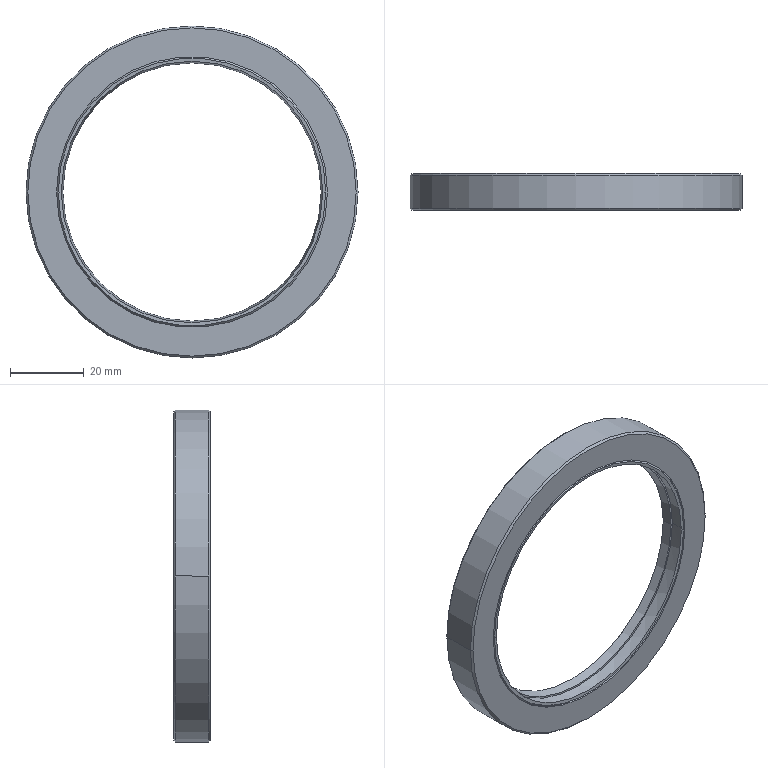Part | SolidWorks | features BaseBody 1 | 1 solid | 37 faces | box 90 x 10 x 90 mm | volume 7063 mm3 | cone 20 | cylinder 8 | plane 5 | spline 4 | commonest cylinder face diameters 73.436 x4 88 x2 90 x2
STEP:
#1=CARTESIAN_POINT('',(36.965,3.733,0.));
#2=VERTEX_POINT('',#1);
#3=CARTESIAN_POINT('',(-36.965,3.733,0.));
#4=VERTEX_POINT('',#3);
#5=CARTESIAN_POINT('',(0.,3.733,0.));
#6=DIRECTION('',(0.,1.,0.));
#7=DIRECTION('',(-1.,0.,0.));
#8=AXIS2_PLACEMENT_3D('',#5,#6,#7);
#9=CIRCLE('',#8,36.965);
#10=EDGE_CURVE('',#2,#4,#9,.T.);
#11=ORIENTED_EDGE('',*,*,#10,.F.);
#12=CARTESIAN_POINT('',(36.518,3.286,0.));
#13=VERTEX_POINT('',#12);
#14=CARTESIAN_POINT('',(36.518,3.733,0.));
#15=DIRECTION('',(0.,0.,-1.));
#16=DIRECTION('',(1.,0.,0.));
#17=AXIS2_PLACEMENT_3D('',#14,#15,#16);
#18=CIRCLE('',#17,0.4472);
#19=EDGE_CURVE('',#2,#13,#18,.T.);
#20=ORIENTED_EDGE('',*,*,#19,.T.);
#21=CARTESIAN_POINT('',(-36.518,3.286,0.));
#22=VERTEX_POINT('',#21);
#23=CARTESIAN_POINT('',(0.,3.286,0.));
#24=DIRECTION('',(0.,-1.,0.));
#25=DIRECTION('',(1.,0.,0.));
#26=AXIS2_PLACEMENT_3D('',#23,#24,#25);
#27=CIRCLE('',#26,36.518);
#28=EDGE_CURVE('',#22,#13,#27,.T.);
#29=ORIENTED_EDGE('',*,*,#28,.F.);
#30=CARTESIAN_POINT('',(-36.518,3.733,0.));
#31=DIRECTION('',(0.,0.,1.));
#32=DIRECTION('',(-1.,0.,0.));
#33=AXIS2_PLACEMENT_3D('',#30,#31,#32);
#34=CIRCLE('',#33,0.4472);
#35=EDGE_CURVE('',#4,#22,#34,.T.);
#36=ORIENTED_EDGE('',*,*,#35,.F.);
#37=EDGE_LOOP('',(#11,#20,#29,#36));
#38=FACE_OUTER_BOUND('',#37,.T.);
#39=CARTESIAN_POINT('',(36.965,3.733,0.));
#40=CARTESIAN_POINT('',(36.965,3.733,-73.93));
#41=CARTESIAN_POINT('',(-36.965,3.733,-73.93));
#42=CARTESIAN_POINT('',(-36.965,3.733,0.));
#43=CARTESIAN_POINT('',(36.965,3.471,0.));
#44=CARTESIAN_POINT('',(36.965,3.471,-73.93));
#45=CARTESIAN_POINT('',(-36.965,3.471,-73.93));
#46=CARTESIAN_POINT('',(-36.965,3.471,0.));
#47=CARTESIAN_POINT('',(36.78,3.286,0.));
#48=CARTESIAN_POINT('',(36.78,3.286,-73.56));
#49=CARTESIAN_POINT('',(-36.78,3.286,-73.56));
#50=CARTESIAN_POINT('',(-36.78,3.286,0.));
#51=CARTESIAN_POINT('',(36.518,3.286,0.));
#52=CARTESIAN_POINT('',(36.518,3.286,-73.036));
#53=CARTESIAN_POINT('',(-36.518,3.286,-73.036));
#54=CARTESIAN_POINT('',(-36.518,3.286,0.));
#55=(BOUNDED_SURFACE()B_SPLINE_SURFACE(3,3,((#39,#40,#41,#42),(#43,#44,#45,#46),(#47,#48,#49,#50),(#51,#52,#53,#54)),.UNSPECIFIED.,.F.,.F.,.F.)B_SPLINE_SURFACE_WITH_KNOTS((4,4),(4,4),(0.,1.),(0.,1.),.UNSPECIFIED.)GEOMETRIC_REPRESENTATION_ITEM()RATIONAL_B_SPLINE_SURFACE(((1.,0.3333,0.3333,1.),(0.8047,0.2682,0.2682,0.8047),(0.8047,0.2682,0.2682,0.8047),(1.,0.3333,0.3333,1.)))REPRESENTATION_ITEM('')SURFACE());
#56=ADVANCED_FACE('',(#38),#55,.T.);
#57=CARTESIAN_POINT('',(-36.718,4.133,0.));
#58=VERTEX_POINT('',#57);
#59=CARTESIAN_POINT('',(36.718,4.133,0.));
#60=VERTEX_POINT('',#59);
#61=CARTESIAN_POINT('',(0.,4.133,0.));
#62=DIRECTION('',(0.,-1.,0.));
#63=DIRECTION('',(-1.,0.,0.));
#64=AXIS2_PLACEMENT_3D('',#61,#62,#63);
#65=CIRCLE('',#64,36.718);
#66=EDGE_CURVE('',#58,#60,#65,.T.);
#67=ORIENTED_EDGE('',*,*,#66,.T.);
#68=CARTESIAN_POINT('',(36.518,3.733,0.));
#69=DIRECTION('',(0.,0.,-1.));
#70=DIRECTION('',(1.,0.,0.));
#71=AXIS2_PLACEMENT_3D('',#68,#69,#70);
#72=CIRCLE('',#71,0.4472);
#73=EDGE_CURVE('',#60,#2,#72,.T.);
#74=ORIENTED_EDGE('',*,*,#73,.T.);
#75=ORIENTED_EDGE('',*,*,#10,.T.);
#76=CARTESIAN_POINT('',(-36.518,3.733,0.));
#77=DIRECTION('',(0.,0.,1.));
#78=DIRECTION('',(-1.,0.,0.));
#79=AXIS2_PLACEMENT_3D('',#76,#77,#78);
#80=CIRCLE('',#79,0.4472);
#81=EDGE_CURVE('',#58,#4,#80,.T.);
#82=ORIENTED_EDGE('',*,*,#81,.F.);
#83=EDGE_LOOP('',(#67,#74,#75,#82));
#84=FACE_OUTER_BOUND('',#83,.T.);
#85=CARTESIAN_POINT('',(36.718,4.133,0.));
#86=CARTESIAN_POINT('',(36.718,4.133,-73.436));
#87=CARTESIAN_POINT('',(-36.718,4.133,-73.436));
#88=CARTESIAN_POINT('',(-36.718,4.133,0.));
#89=CARTESIAN_POINT('',(36.873,4.055,0.));
#90=CARTESIAN_POINT('',(36.873,4.055,-73.747));
#91=CARTESIAN_POINT('',(-36.873,4.055,-73.747));
#92=CARTESIAN_POINT('',(-36.873,4.055,0.));
#93=CARTESIAN_POINT('',(36.965,3.907,0.));
#94=CARTESIAN_POINT('',(36.965,3.907,-73.93));
#95=CARTESIAN_POINT('',(-36.965,3.907,-73.93));
#96=CARTESIAN_POINT('',(-36.965,3.907,0.));
#97=CARTESIAN_POINT('',(36.965,3.733,0.));
#98=CARTESIAN_POINT('',(36.965,3.733,-73.93));
#99=CARTESIAN_POINT('',(-36.965,3.733,-73.93));
#100=CARTESIAN_POINT('',(-36.965,3.733,0.));
#101=(BOUNDED_SURFACE()B_SPLINE_SURFACE(3,3,((#85,#86,#87,#88),(#89,#90,#91,#92),(#93,#94,#95,#96),(#97,#98,#99,#100)),.UNSPECIFIED.,.F.,.F.,.T.)B_SPLINE_SURFACE_WITH_KNOTS((4,4),(4,4),(0.,1.),(0.,1.),.UNSPECIFIED.)GEOMETRIC_REPRESENTATION_ITEM()RATIONAL_B_SPLINE_SURFACE(((1.,0.3333,0.3333,1.),(0.9004,0.3001,0.3001,0.9004),(0.9004,0.3001,0.3001,0.9004),(1.,0.3333,0.3333,1.)))REPRESENTATION_ITEM('')SURFACE());
#102=ADVANCED_FACE('',(#84),#101,.T.);
#103=CARTESIAN_POINT('',(44.5,0.,0.));
#104=VERTEX_POINT('',#103);
#105=CARTESIAN_POINT('',(-44.5,0.,0.));
#106=VERTEX_POINT('',#105);
#107=CARTESIAN_POINT('',(0.,0.,0.));
#108=DIRECTION('',(0.,-1.,0.));
#109=DIRECTION('',(-1.,0.,0.));
#110=AXIS2_PLACEMENT_3D('',#107,#108,#109);
#111=CIRCLE('',#110,44.5);
#112=EDGE_CURVE('',#104,#106,#111,.T.);
#113=ORIENTED_EDGE('',*,*,#112,.F.);
#114=CARTESIAN_POINT('',(45.,0.5,0.));
#115=VERTEX_POINT('',#114);
#116=CARTESIAN_POINT('',(45.,0.5,0.));
#117=DIRECTION('',(0.7071,0.7071,0.));
#118=VECTOR('',#117,1000.);
#119=LINE('',#116,#118);
#120=EDGE_CURVE('',#104,#115,#119,.T.);
#121=ORIENTED_EDGE('',*,*,#120,.T.);
#122=CARTESIAN_POINT('',(-45.,0.5,0.));
#123=VERTEX_POINT('',#122);
#124=CARTESIAN_POINT('',(0.,0.5,0.));
#125=DIRECTION('',(0.,-1.,0.));
#126=DIRECTION('',(-1.,0.,0.));
#127=AXIS2_PLACEMENT_3D('',#124,#125,#126);
#128=CIRCLE('',#127,45.);
#129=EDGE_CURVE('',#115,#123,#128,.T.);
#130=ORIENTED_EDGE('',*,*,#129,.T.);
#131=CARTESIAN_POINT('',(-45.,0.5,0.));
#132=DIRECTION('',(-0.7071,0.7071,0.));
#133=VECTOR('',#132,1000.);
#134=LINE('',#131,#133);
#135=EDGE_CURVE('',#106,#123,#134,.T.);
#136=ORIENTED_EDGE('',*,*,#135,.F.);
#137=EDGE_LOOP('',(#113,#121,#130,#136));
#138=FACE_OUTER_BOUND('',#137,.T.);
#139=CARTESIAN_POINT('',(0.,0.5,0.));
#140=DIRECTION('',(0.,1.,0.));
#141=DIRECTION('',(-1.,0.,0.));
#142=AXIS2_PLACEMENT_3D('',#139,#140,#141);
#143=CONICAL_SURFACE('',#142,45.,0.7854);
#144=ADVANCED_FACE('',(#138),#143,.T.);
#145=CARTESIAN_POINT('',(36.718,0.,0.));
#146=VERTEX_POINT('',#145);
#147=CARTESIAN_POINT('',(-36.718,0.,0.));
#148=VERTEX_POINT('',#147);
#149=CARTESIAN_POINT('',(0.,0.,0.));
#150=DIRECTION('',(0.,1.,0.));
#151=DIRECTION('',(-1.,0.,0.));
#152=AXIS2_PLACEMENT_3D('',#149,#150,#151);
#153=CIRCLE('',#152,36.718);
#154=EDGE_CURVE('',#146,#148,#153,.T.);
#155=ORIENTED_EDGE('',*,*,#154,.F.);
#156=CARTESIAN_POINT('',(36.718,0.5,0.));
#157=VERTEX_POINT('',#156);
#158=CARTESIAN_POINT('',(36.718,5.977,0.));
#159=DIRECTION('',(0.,1.,0.));
#160=VECTOR('',#159,1000.);
#161=LINE('',#158,#160);
#162=EDGE_CURVE('',#146,#157,#161,.T.);
#163=ORIENTED_EDGE('',*,*,#162,.T.);
#164=CARTESIAN_POINT('',(-36.718,0.5,0.));
#165=VERTEX_POINT('',#164);
#166=CARTESIAN_POINT('',(0.,0.5,0.));
#167=DIRECTION('',(0.,-1.,0.));
#168=DIRECTION('',(-1.,0.,0.));
#169=AXIS2_PLACEMENT_3D('',#166,#167,#168);
#170=CIRCLE('',#169,36.718);
#171=EDGE_CURVE('',#165,#157,#170,.T.);
#172=ORIENTED_EDGE('',*,*,#171,.F.);
#173=CARTESIAN_POINT('',(-36.718,5.977,0.));
#174=DIRECTION('',(0.,1.,0.));
#175=VECTOR('',#174,1000.);
#176=LINE('',#173,#175);
#177=EDGE_CURVE('',#148,#165,#176,.T.);
#178=ORIENTED_EDGE('',*,*,#177,.F.);
#179=EDGE_LOOP('',(#155,#163,#172,#178));
#180=FACE_OUTER_BOUND('',#179,.T.);
#181=CARTESIAN_POINT('',(0.,5.977,0.));
#182=DIRECTION('',(0.,1.,0.));
#183=DIRECTION('',(-1.,0.,0.));
#184=AXIS2_PLACEMENT_3D('',#181,#182,#183);
#185=CYLINDRICAL_SURFACE('',#184,36.718);
#186=ADVANCED_FACE('',(#180),#185,.F.);
#187=ORIENTED_EDGE('',*,*,#129,.F.);
#188=CARTESIAN_POINT('',(45.,9.5,0.));
#189=VERTEX_POINT('',#188);
#190=CARTESIAN_POINT('',(45.,5.977,0.));
#191=DIRECTION('',(0.,1.,0.));
#192=VECTOR('',#191,1000.);
#193=LINE('',#190,#192);
#194=EDGE_CURVE('',#115,#189,#193,.T.);
#195=ORIENTED_EDGE('',*,*,#194,.T.);
#196=CARTESIAN_POINT('',(-45.,9.5,0.));
#197=VERTEX_POINT('',#196);
#198=CARTESIAN_POINT('',(0.,9.5,0.));
#199=DIRECTION('',(0.,-1.,0.));
#200=DIRECTION('',(-1.,0.,0.));
#201=AXIS2_PLACEMENT_3D('',#198,#199,#200);
#202=CIRCLE('',#201,45.);
#203=EDGE_CURVE('',#189,#197,#202,.T.);
#204=ORIENTED_EDGE('',*,*,#203,.T.);
#205=CARTESIAN_POINT('',(-45.,5.977,0.));
#206=DIRECTION('',(0.,1.,0.));
#207=VECTOR('',#206,1000.);
#208=LINE('',#205,#207);
#209=EDGE_CURVE('',#123,#197,#208,.T.);
#210=ORIENTED_EDGE('',*,*,#209,.F.);
#211=EDGE_LOOP('',(#187,#195,#204,#210));
#212=FACE_OUTER_BOUND('',#211,.T.);
#213=CARTESIAN_POINT('',(0.,5.977,0.));
#214=DIRECTION('',(0.,1.,0.));
#215=DIRECTION('',(-1.,0.,0.));
#216=AXIS2_PLACEMENT_3D('',#213,#214,#215);
#217=CYLINDRICAL_SURFACE('',#216,45.);
#218=ADVANCED_FACE('',(#212),#217,.T.);
#219=CARTESIAN_POINT('',(-36.26,0.,0.));
#220=VERTEX_POINT('',#219);
#221=CARTESIAN_POINT('',(36.26,0.,0.));
#222=VERTEX_POINT('',#221);
#223=CARTESIAN_POINT('',(0.,0.,0.));
#224=DIRECTION('',(0.,1.,0.));
#225=DIRECTION('',(-1.,0.,0.));
#226=AXIS2_PLACEMENT_3D('',#223,#224,#225);
#227=CIRCLE('',#226,36.26);
#228=EDGE_CURVE('',#220,#222,#227,.T.);
#229=ORIENTED_EDGE('',*,*,#228,.T.);
#230=CARTESIAN_POINT('',(36.718,0.5,0.));
#231=DIRECTION('',(0.6756,0.7373,0.));
#232=VECTOR('',#231,1000.);
#233=LINE('',#230,#232);
#234=EDGE_CURVE('',#222,#157,#233,.T.);
#235=ORIENTED_EDGE('',*,*,#234,.T.);
#236=CARTESIAN_POINT('',(0.,0.5,0.));
#237=DIRECTION('',(0.,-1.,0.));
#238=DIRECTION('',(-1.,0.,0.));
#239=AXIS2_PLACEMENT_3D('',#236,#237,#238);
#240=CIRCLE('',#239,36.718);
#241=EDGE_CURVE('',#157,#165,#240,.T.);
#242=ORIENTED_EDGE('',*,*,#241,.T.);
#243=CARTESIAN_POINT('',(-36.718,0.5,0.));
#244=DIRECTION('',(-0.6756,0.7373,0.));
#245=VECTOR('',#244,1000.);
#246=LINE('',#243,#245);
#247=EDGE_CURVE('',#220,#165,#246,.T.);
#248=ORIENTED_EDGE('',*,*,#247,.F.);
#249=EDGE_LOOP('',(#229,#235,#242,#248));
#250=FACE_OUTER_BOUND('',#249,.T.);
#251=CARTESIAN_POINT('',(0.,0.5,0.));
#252=DIRECTION('',(0.,1.,0.));
#253=DIRECTION('',(-1.,0.,0.));
#254=AXIS2_PLACEMENT_3D('',#251,#252,#253);
#255=CONICAL_SURFACE('',#254,36.718,0.7418);
#256=ADVANCED_FACE('',(#250),#255,.T.);
#257=CARTESIAN_POINT('',(44.5,10.,0.));
#258=VERTEX_POINT('',#257);
#259=CARTESIAN_POINT('',(-44.5,10.,0.));
#260=VERTEX_POINT('',#259);
#261=CARTESIAN_POINT('',(0.,10.,0.));
#262=DIRECTION('',(0.,-1.,0.));
#263=DIRECTION('',(1.,0.,0.));
#264=AXIS2_PLACEMENT_3D('',#261,#262,#263);
#265=CIRCLE('',#264,44.5);
#266=EDGE_CURVE('',#258,#260,#265,.T.);
#267=ORIENTED_EDGE('',*,*,#266,.T.);
#268=CARTESIAN_POINT('',(-45.,9.5,0.));
#269=DIRECTION('',(-0.7071,-0.7071,0.));
#270=VECTOR('',#269,1000.);
#271=LINE('',#268,#270);
#272=EDGE_CURVE('',#260,#197,#271,.T.);
#273=ORIENTED_EDGE('',*,*,#272,.T.);
#274=ORIENTED_EDGE('',*,*,#203,.F.);
#275=CARTESIAN_POINT('',(45.,9.5,0.));
#276=DIRECTION('',(0.7071,-0.7071,0.));
#277=VECTOR('',#276,1000.);
#278=LINE('',#275,#277);
#279=EDGE_CURVE('',#258,#189,#278,.T.);
#280=ORIENTED_EDGE('',*,*,#279,.F.);
#281=EDGE_LOOP('',(#267,#273,#274,#280));
#282=FACE_OUTER_BOUND('',#281,.T.);
#283=CARTESIAN_POINT('',(0.,9.5,0.));
#284=DIRECTION('',(0.,-1.,0.));
#285=DIRECTION('',(1.,0.,0.));
#286=AXIS2_PLACEMENT_3D('',#283,#284,#285);
#287=CONICAL_SURFACE('',#286,45.,0.7854);
#288=ADVANCED_FACE('',(#282),#287,.T.);
#289=CARTESIAN_POINT('',(-35.453,0.07053,0.));
#290=VERTEX_POINT('',#289);
#291=CARTESIAN_POINT('',(35.453,0.07053,0.));
#292=VERTEX_POINT('',#291);
#293=CARTESIAN_POINT('',(0.,0.07053,0.));
#294=DIRECTION('',(0.,-1.,0.));
#295=DIRECTION('',(1.,0.,0.));
#296=AXIS2_PLACEMENT_3D('',#293,#294,#295);
#297=CIRCLE('',#296,35.453);
#298=EDGE_CURVE('',#290,#292,#297,.T.);
#299=ORIENTED_EDGE('',*,*,#298,.F.);
#300=CARTESIAN_POINT('',(-36.26,0.,0.));
#301=DIRECTION('',(-0.9962,-0.08716,0.));
#302=VECTOR('',#301,1000.);
#303=LINE('',#300,#302);
#304=EDGE_CURVE('',#290,#220,#303,.T.);
#305=ORIENTED_EDGE('',*,*,#304,.T.);
#306=CARTESIAN_POINT('',(0.,0.,0.));
#307=DIRECTION('',(0.,1.,0.));
#308=DIRECTION('',(-1.,0.,0.));
#309=AXIS2_PLACEMENT_3D('',#306,#307,#308);
#310=CIRCLE('',#309,36.26);
#311=EDGE_CURVE('',#222,#220,#310,.T.);
#312=ORIENTED_EDGE('',*,*,#311,.F.);
#313=CARTESIAN_POINT('',(36.26,0.,0.));
#314=DIRECTION('',(0.9962,-0.08716,0.));
#315=VECTOR('',#314,1000.);
#316=LINE('',#313,#315);
#317=EDGE_CURVE('',#292,#222,#316,.T.);
#318=ORIENTED_EDGE('',*,*,#317,.F.);
#319=EDGE_LOOP('',(#299,#305,#312,#318));
#320=FACE_OUTER_BOUND('',#319,.T.);
#321=CARTESIAN_POINT('',(0.,0.,0.));
#322=DIRECTION('',(0.,-1.,0.));
#323=DIRECTION('',(1.,0.,0.));
#324=AXIS2_PLACEMENT_3D('',#321,#322,#323);
#325=CONICAL_SURFACE('',#324,36.26,1.484);
#326=ADVANCED_FACE('',(#320),#325,.F.);
#327=ORIENTED_EDGE('',*,*,#298,.T.);
#328=CARTESIAN_POINT('',(36.26,0.5,0.));
#329=VERTEX_POINT('',#328);
#330=CARTESIAN_POINT('',(36.26,0.5,0.));
#331=DIRECTION('',(0.8826,0.4702,0.));
#332=VECTOR('',#331,1000.);
#333=LINE('',#330,#332);
#334=EDGE_CURVE('',#292,#329,#333,.T.);
#335=ORIENTED_EDGE('',*,*,#334,.T.);
#336=CARTESIAN_POINT('',(-36.26,0.5,0.));
#337=VERTEX_POINT('',#336);
#338=CARTESIAN_POINT('',(0.,0.5,0.));
#339=DIRECTION('',(0.,-1.,0.));
#340=DIRECTION('',(-1.,0.,0.));
#341=AXIS2_PLACEMENT_3D('',#338,#339,#340);
#342=CIRCLE('',#341,36.26);
#343=EDGE_CURVE('',#337,#329,#342,.T.);
#344=ORIENTED_EDGE('',*,*,#343,.F.);
#345=CARTESIAN_POINT('',(-36.26,0.5,0.));
#346=DIRECTION('',(-0.8826,0.4702,0.));
#347=VECTOR('',#346,1000.);
#348=LINE('',#345,#347);
#349=EDGE_CURVE('',#290,#337,#348,.T.);
#350=ORIENTED_EDGE('',*,*,#349,.F.);
#351=EDGE_LOOP('',(#327,#335,#344,#350));
#352=FACE_OUTER_BOUND('',#351,.T.);
#353=CARTESIAN_POINT('',(0.,0.5,0.));
#354=DIRECTION('',(0.,1.,0.));
#355=DIRECTION('',(-1.,0.,0.));
#356=AXIS2_PLACEMENT_3D('',#353,#354,#355);
#357=CONICAL_SURFACE('',#356,36.26,1.081);
#358=ADVANCED_FACE('',(#352),#357,.F.);
#359=CARTESIAN_POINT('',(44.,9.5,0.));
#360=VERTEX_POINT('',#359);
#361=CARTESIAN_POINT('',(-44.,9.5,0.));
#362=VERTEX_POINT('',#361);
#363=CARTESIAN_POINT('',(0.,9.5,0.));
#364=DIRECTION('',(0.,1.,0.));
#365=DIRECTION('',(-1.,0.,0.));
#366=AXIS2_PLACEMENT_3D('',#363,#364,#365);
#367=CIRCLE('',#366,44.);
#368=EDGE_CURVE('',#360,#362,#367,.T.);
#369=ORIENTED_EDGE('',*,*,#368,.F.);
#370=CARTESIAN_POINT('',(44.,10.,0.));
#371=VERTEX_POINT('',#370);
#372=CARTESIAN_POINT('',(44.,5.977,0.));
#373=DIRECTION('',(0.,1.,0.));
#374=VECTOR('',#373,1000.);
#375=LINE('',#372,#374);
#376=EDGE_CURVE('',#360,#371,#375,.T.);
#377=ORIENTED_EDGE('',*,*,#376,.T.);
#378=CARTESIAN_POINT('',(-44.,10.,0.));
#379=VERTEX_POINT('',#378);
#380=CARTESIAN_POINT('',(0.,10.,0.));
#381=DIRECTION('',(0.,-1.,0.));
#382=DIRECTION('',(-1.,0.,0.));
#383=AXIS2_PLACEMENT_3D('',#380,#381,#382);
#384=CIRCLE('',#383,44.);
#385=EDGE_CURVE('',#379,#371,#384,.T.);
#386=ORIENTED_EDGE('',*,*,#385,.F.);
#387=CARTESIAN_POINT('',(-44.,5.977,0.));
#388=DIRECTION('',(0.,1.,0.));
#389=VECTOR('',#388,1000.);
#390=LINE('',#387,#389);
#391=EDGE_CURVE('',#362,#379,#390,.T.);
#392=ORIENTED_EDGE('',*,*,#391,.F.);
#393=EDGE_LOOP('',(#369,#377,#386,#392));
#394=FACE_OUTER_BOUND('',#393,.T.);
#395=CARTESIAN_POINT('',(0.,5.977,0.));
#396=DIRECTION('',(0.,1.,0.));
#397=DIRECTION('',(-1.,0.,0.));
#398=AXIS2_PLACEMENT_3D('',#395,#396,#397);
#399=CYLINDRICAL_SURFACE('',#398,44.);
#400=ADVANCED_FACE('',(#394),#399,.F.);
#401=CARTESIAN_POINT('',(-35.953,4.,0.));
#402=VERTEX_POINT('',#401);
#403=CARTESIAN_POINT('',(35.953,4.,0.));
#404=VERTEX_POINT('',#403);
#405=CARTESIAN_POINT('',(0.,4.,0.));
#406=DIRECTION('',(0.,-1.,0.));
#407=DIRECTION('',(1.,0.,0.));
#408=AXIS2_PLACEMENT_3D('',#405,#406,#407);
#409=CIRCLE('',#408,35.953);
#410=EDGE_CURVE('',#402,#404,#409,.T.);
#411=ORIENTED_EDGE('',*,*,#410,.F.);
#412=CARTESIAN_POINT('',(-36.26,0.5,0.));
#413=DIRECTION('',(-0.08716,-0.9962,0.));
#414=VECTOR('',#413,1000.);
#415=LINE('',#412,#414);
#416=EDGE_CURVE('',#402,#337,#415,.T.);
#417=ORIENTED_EDGE('',*,*,#416,.T.);
#418=ORIENTED_EDGE('',*,*,#343,.T.);
#419=CARTESIAN_POINT('',(36.26,0.5,0.));
#420=DIRECTION('',(0.08716,-0.9962,0.));
#421=VECTOR('',#420,1000.);
#422=LINE('',#419,#421);
#423=EDGE_CURVE('',#404,#329,#422,.T.);
#424=ORIENTED_EDGE('',*,*,#423,.F.);
#425=EDGE_LOOP('',(#411,#417,#418,#424));
#426=FACE_OUTER_BOUND('',#425,.T.);
#427=CARTESIAN_POINT('',(0.,0.5,0.));
#428=DIRECTION('',(0.,-1.,0.));
#429=DIRECTION('',(1.,0.,0.));
#430=AXIS2_PLACEMENT_3D('',#427,#428,#429);
#431=CONICAL_SURFACE('',#430,36.26,0.08727);
#432=ADVANCED_FACE('',(#426),#431,.F.);
#433=CARTESIAN_POINT('',(43.256,1.,0.));
#434=VERTEX_POINT('',#433);
#435=CARTESIAN_POINT('',(-43.256,1.,0.));
#436=VERTEX_POINT('',#435);
#437=CARTESIAN_POINT('',(0.,1.,0.));
#438=DIRECTION('',(0.,1.,0.));
#439=DIRECTION('',(-1.,0.,0.));
#440=AXIS2_PLACEMENT_3D('',#437,#438,#439);
#441=CIRCLE('',#440,43.256);
#442=EDGE_CURVE('',#434,#436,#441,.T.);
#443=ORIENTED_EDGE('',*,*,#442,.F.);
#444=CARTESIAN_POINT('',(44.,9.5,0.));
#445=DIRECTION('',(0.08716,0.9962,0.));
#446=VECTOR('',#445,1000.);
#447=LINE('',#444,#446);
#448=EDGE_CURVE('',#434,#360,#447,.T.);
#449=ORIENTED_EDGE('',*,*,#448,.T.);
#450=ORIENTED_EDGE('',*,*,#368,.T.);
#451=CARTESIAN_POINT('',(-44.,9.5,0.));
#452=DIRECTION('',(-0.08716,0.9962,0.));
#453=VECTOR('',#452,1000.);
#454=LINE('',#451,#453);
#455=EDGE_CURVE('',#436,#362,#454,.T.);
#456=ORIENTED_EDGE('',*,*,#455,.F.);
#457=EDGE_LOOP('',(#443,#449,#450,#456));
#458=FACE_OUTER_BOUND('',#457,.T.);
#459=CARTESIAN_POINT('',(0.,9.5,0.));
#460=DIRECTION('',(0.,1.,0.));
#461=DIRECTION('',(-1.,0.,0.));
#462=AXIS2_PLACEMENT_3D('',#459,#460,#461);
#463=CONICAL_SURFACE('',#462,44.,0.08727);
#464=ADVANCED_FACE('',(#458),#463,.F.);
#465=CARTESIAN_POINT('',(-35.,6.571,0.));
#466=VERTEX_POINT('',#465);
#467=CARTESIAN_POINT('',(35.,6.571,0.));
#468=VERTEX_POINT('',#467);
#469=CARTESIAN_POINT('',(0.,6.571,0.));
#470=DIRECTION('',(0.,-1.,0.));
#471=DIRECTION('',(1.,0.,0.));
#472=AXIS2_PLACEMENT_3D('',#469,#470,#471);
#473=CIRCLE('',#472,35.);
#474=EDGE_CURVE('',#466,#468,#473,.T.);
#475=ORIENTED_EDGE('',*,*,#474,.F.);
#476=CARTESIAN_POINT('',(-35.453,4.,0.));
#477=VERTEX_POINT('',#476);
#478=CARTESIAN_POINT('',(-35.453,4.,0.));
#479=DIRECTION('',(-0.1736,-0.9848,0.));
#480=VECTOR('',#479,1000.);
#481=LINE('',#478,#480);
#482=EDGE_CURVE('',#466,#477,#481,.T.);
#483=ORIENTED_EDGE('',*,*,#482,.T.);
#484=CARTESIAN_POINT('',(35.453,4.,0.));
#485=VERTEX_POINT('',#484);
#486=CARTESIAN_POINT('',(0.,4.,0.));
#487=DIRECTION('',(0.,1.,0.));
#488=DIRECTION('',(1.,0.,0.));
#489=AXIS2_PLACEMENT_3D('',#486,#487,#488);
#490=CIRCLE('',#489,35.453);
#491=EDGE_CURVE('',#485,#477,#490,.T.);
#492=ORIENTED_EDGE('',*,*,#491,.F.);
#493=CARTESIAN_POINT('',(35.453,4.,0.));
#494=DIRECTION('',(0.1736,-0.9848,0.));
#495=VECTOR('',#494,1000.);
#496=LINE('',#493,#495);
#497=EDGE_CURVE('',#468,#485,#496,.T.);
#498=ORIENTED_EDGE('',*,*,#497,.F.);
#499=EDGE_LOOP('',(#475,#483,#492,#498));
#500=FACE_OUTER_BOUND('',#499,.T.);
#501=CARTESIAN_POINT('',(0.,4.,0.));
#502=DIRECTION('',(0.,-1.,0.));
#503=DIRECTION('',(1.,0.,0.));
#504=AXIS2_PLACEMENT_3D('',#501,#502,#503);
#505=CONICAL_SURFACE('',#504,35.453,0.1745);
#506=ADVANCED_FACE('',(#500),#505,.F.);
#507=CARTESIAN_POINT('',(0.,3.286,0.));
#508=DIRECTION('',(0.,-1.,0.));
#509=DIRECTION('',(1.,0.,0.));
#510=AXIS2_PLACEMENT_3D('',#507,#508,#509);
#511=CIRCLE('',#510,36.518);
#512=EDGE_CURVE('',#13,#22,#511,.T.);
#513=ORIENTED_EDGE('',*,*,#512,.T.);
#514=CARTESIAN_POINT('',(-36.718,1.,0.));
#515=VERTEX_POINT('',#514);
#516=CARTESIAN_POINT('',(-36.718,1.,0.));
#517=DIRECTION('',(-0.08716,-0.9962,0.));
#518=VECTOR('',#517,1000.);
#519=LINE('',#516,#518);
#520=EDGE_CURVE('',#22,#515,#519,.T.);
#521=ORIENTED_EDGE('',*,*,#520,.T.);
#522=CARTESIAN_POINT('',(36.718,1.,0.));
#523=VERTEX_POINT('',#522);
#524=CARTESIAN_POINT('',(0.,1.,0.));
#525=DIRECTION('',(0.,-1.,0.));
#526=DIRECTION('',(1.,0.,0.));
#527=AXIS2_PLACEMENT_3D('',#524,#525,#526);
#528=CIRCLE('',#527,36.718);
#529=EDGE_CURVE('',#523,#515,#528,.T.);
#530=ORIENTED_EDGE('',*,*,#529,.F.);
#531=CARTESIAN_POINT('',(36.718,1.,0.));
#532=DIRECTION('',(0.08716,-0.9962,0.));
#533=VECTOR('',#532,1000.);
#534=LINE('',#531,#533);
#535=EDGE_CURVE('',#13,#523,#534,.T.);
#536=ORIENTED_EDGE('',*,*,#535,.F.);
#537=EDGE_LOOP('',(#513,#521,#530,#536));
#538=FACE_OUTER_BOUND('',#537,.T.);
#539=CARTESIAN_POINT('',(0.,1.,0.));
#540=DIRECTION('',(0.,-1.,0.));
#541=DIRECTION('',(1.,0.,0.));
#542=AXIS2_PLACEMENT_3D('',#539,#540,#541);
#543=CONICAL_SURFACE('',#542,36.718,0.08727);
#544=ADVANCED_FACE('',(#538),#543,.T.);
#545=ORIENTED_EDGE('',*,*,#474,.T.);
#546=CARTESIAN_POINT('',(36.224,7.429,0.));
#547=VERTEX_POINT('',#546);
#548=CARTESIAN_POINT('',(36.224,7.429,0.));
#549=DIRECTION('',(0.8192,0.5736,0.));
#550=VECTOR('',#549,1000.);
#551=LINE('',#548,#550);
#552=EDGE_CURVE('',#468,#547,#551,.T.);
#553=ORIENTED_EDGE('',*,*,#552,.T.);
#554=CARTESIAN_POINT('',(-36.224,7.429,0.));
#555=VERTEX_POINT('',#554);
#556=CARTESIAN_POINT('',(0.,7.429,0.));
#557=DIRECTION('',(0.,-1.,0.));
#558=DIRECTION('',(-1.,0.,0.));
#559=AXIS2_PLACEMENT_3D('',#556,#557,#558);
#560=CIRCLE('',#559,36.224);
#561=EDGE_CURVE('',#555,#547,#560,.T.);
#562=ORIENTED_EDGE('',*,*,#561,.F.);
#563=CARTESIAN_POINT('',(-36.224,7.429,0.));
#564=DIRECTION('',(-0.8192,0.5736,0.));
#565=VECTOR('',#564,1000.);
#566=LINE('',#563,#565);
#567=EDGE_CURVE('',#466,#555,#566,.T.);
#568=ORIENTED_EDGE('',*,*,#567,.F.);
#569=EDGE_LOOP('',(#545,#553,#562,#568));
#570=FACE_OUTER_BOUND('',#569,.T.);
#571=CARTESIAN_POINT('',(0.,7.429,0.));
#572=DIRECTION('',(0.,1.,0.));
#573=DIRECTION('',(-1.,0.,0.));
#574=AXIS2_PLACEMENT_3D('',#571,#572,#573);
#575=CONICAL_SURFACE('',#574,36.224,0.9599);
#576=ADVANCED_FACE('',(#570),#575,.F.);
#577=ORIENTED_EDGE('',*,*,#73,.F.);
#578=CARTESIAN_POINT('',(0.,4.133,0.));
#579=DIRECTION('',(0.,-1.,0.));
#580=DIRECTION('',(-1.,0.,0.));
#581=AXIS2_PLACEMENT_3D('',#578,#579,#580);
#582=CIRCLE('',#581,36.718);
#583=EDGE_CURVE('',#60,#58,#582,.T.);
#584=ORIENTED_EDGE('',*,*,#583,.T.);
#585=ORIENTED_EDGE('',*,*,#81,.T.);
#586=CARTESIAN_POINT('',(0.,3.733,0.));
#587=DIRECTION('',(0.,1.,0.));
#588=DIRECTION('',(-1.,0.,0.));
#589=AXIS2_PLACEMENT_3D('',#586,#587,#588);
#590=CIRCLE('',#589,36.965);
#591=EDGE_CURVE('',#4,#2,#590,.T.);
#592=ORIENTED_EDGE('',*,*,#591,.T.);
#593=EDGE_LOOP('',(#577,#584,#585,#592));
#594=FACE_OUTER_BOUND('',#593,.T.);
#595=CARTESIAN_POINT('',(-36.718,4.133,0.));
#596=CARTESIAN_POINT('',(-36.718,4.133,73.436));
#597=CARTESIAN_POINT('',(36.718,4.133,73.436));
#598=CARTESIAN_POINT('',(36.718,4.133,0.));
#599=CARTESIAN_POINT('',(-36.873,4.055,0.));
#600=CARTESIAN_POINT('',(-36.873,4.055,73.747));
#601=CARTESIAN_POINT('',(36.873,4.055,73.747));
#602=CARTESIAN_POINT('',(36.873,4.055,0.));
#603=CARTESIAN_POINT('',(-36.965,3.907,0.));
#604=CARTESIAN_POINT('',(-36.965,3.907,73.93));
#605=CARTESIAN_POINT('',(36.965,3.907,73.93));
#606=CARTESIAN_POINT('',(36.965,3.907,0.));
#607=CARTESIAN_POINT('',(-36.965,3.733,0.));
#608=CARTESIAN_POINT('',(-36.965,3.733,73.93));
#609=CARTESIAN_POINT('',(36.965,3.733,73.93));
#610=CARTESIAN_POINT('',(36.965,3.733,0.));
#611=(BOUNDED_SURFACE()B_SPLINE_SURFACE(3,3,((#595,#596,#597,#598),(#599,#600,#601,#602),(#603,#604,#605,#606),(#607,#608,#609,#610)),.UNSPECIFIED.,.F.,.F.,.F.)B_SPLINE_SURFACE_WITH_KNOTS((4,4),(4,4),(0.,1.),(0.,1.),.UNSPECIFIED.)GEOMETRIC_REPRESENTATION_ITEM()RATIONAL_B_SPLINE_SURFACE(((1.,0.3333,0.3333,1.),(0.9004,0.3001,0.3001,0.9004),(0.9004,0.3001,0.3001,0.9004),(1.,0.3333,0.3333,1.)))REPRESENTATION_ITEM('')SURFACE());
#612=ADVANCED_FACE('',(#594),#611,.T.);
#613=ORIENTED_EDGE('',*,*,#583,.F.);
#614=CARTESIAN_POINT('',(36.718,7.429,0.));
#615=VERTEX_POINT('',#614);
#616=CARTESIAN_POINT('',(36.718,5.977,0.));
#617=DIRECTION('',(0.,1.,0.));
#618=VECTOR('',#617,1000.);
#619=LINE('',#616,#618);
#620=EDGE_CURVE('',#60,#615,#619,.T.);
#621=ORIENTED_EDGE('',*,*,#620,.T.);
#622=CARTESIAN_POINT('',(-36.718,7.429,0.));
#623=VERTEX_POINT('',#622);
#624=CARTESIAN_POINT('',(0.,7.429,0.));
#625=DIRECTION('',(0.,1.,0.));
#626=DIRECTION('',(-1.,0.,0.));
#627=AXIS2_PLACEMENT_3D('',#624,#625,#626);
#628=CIRCLE('',#627,36.718);
#629=EDGE_CURVE('',#623,#615,#628,.T.);
#630=ORIENTED_EDGE('',*,*,#629,.F.);
#631=CARTESIAN_POINT('',(-36.718,5.977,0.));
#632=DIRECTION('',(0.,1.,0.));
#633=VECTOR('',#632,1000.);
#634=LINE('',#631,#633);
#635=EDGE_CURVE('',#58,#623,#634,.T.);
#636=ORIENTED_EDGE('',*,*,#635,.F.);
#637=EDGE_LOOP('',(#613,#621,#630,#636));
#638=FACE_OUTER_BOUND('',#637,.T.);
#639=CARTESIAN_POINT('',(0.,5.977,0.));
#640=DIRECTION('',(0.,1.,0.));
#641=DIRECTION('',(-1.,0.,0.));
#642=AXIS2_PLACEMENT_3D('',#639,#640,#641);
#643=CYLINDRICAL_SURFACE('',#642,36.718);
#644=ADVANCED_FACE('',(#638),#643,.T.);
#645=CARTESIAN_POINT('',(0.,0.,0.));
#646=DIRECTION('',(0.,-1.,0.));
#647=DIRECTION('',(-1.,0.,0.));
#648=AXIS2_PLACEMENT_3D('',#645,#646,#647);
#649=CIRCLE('',#648,44.5);
#650=EDGE_CURVE('',#106,#104,#649,.T.);
#651=ORIENTED_EDGE('',*,*,#650,.T.);
#652=ORIENTED_EDGE('',*,*,#112,.T.);
#653=EDGE_LOOP('',(#651,#652));
#654=FACE_OUTER_BOUND('',#653,.T.);
#655=CARTESIAN_POINT('',(0.,0.,0.));
#656=DIRECTION('',(0.,1.,0.));
#657=DIRECTION('',(-1.,0.,0.));
#658=AXIS2_PLACEMENT_3D('',#655,#656,#657);
#659=CIRCLE('',#658,36.718);
#660=EDGE_CURVE('',#148,#146,#659,.T.);
#661=ORIENTED_EDGE('',*,*,#660,.T.);
#662=ORIENTED_EDGE('',*,*,#154,.T.);
#663=EDGE_LOOP('',(#661,#662));
#664=FACE_BOUND('',#663,.T.);
#665=CARTESIAN_POINT('',(-44.5,0.,0.));
#666=DIRECTION('',(0.,-1.,0.));
#667=DIRECTION('',(1.,0.,0.));
#668=AXIS2_PLACEMENT_3D('',#665,#666,#667);
#669=PLANE('',#668);
#670=ADVANCED_FACE('',(#654,#664),#669,.T.);
#671=ORIENTED_EDGE('',*,*,#120,.F.);
#672=ORIENTED_EDGE('',*,*,#650,.F.);
#673=ORIENTED_EDGE('',*,*,#135,.T.);
#674=CARTESIAN_POINT('',(0.,0.5,0.));
#675=DIRECTION('',(0.,-1.,0.));
#676=DIRECTION('',(-1.,0.,0.));
#677=AXIS2_PLACEMENT_3D('',#674,#675,#676);
#678=CIRCLE('',#677,45.);
#679=EDGE_CURVE('',#123,#115,#678,.T.);
#680=ORIENTED_EDGE('',*,*,#679,.T.);
#681=EDGE_LOOP('',(#671,#672,#673,#680));
#682=FACE_OUTER_BOUND('',#681,.T.);
#683=CARTESIAN_POINT('',(0.,0.5,0.));
#684=DIRECTION('',(0.,1.,0.));
#685=DIRECTION('',(-1.,0.,0.));
#686=AXIS2_PLACEMENT_3D('',#683,#684,#685);
#687=CONICAL_SURFACE('',#686,45.,0.7854);
#688=ADVANCED_FACE('',(#682),#687,.T.);
#689=ORIENTED_EDGE('',*,*,#162,.F.);
#690=ORIENTED_EDGE('',*,*,#660,.F.);
#691=ORIENTED_EDGE('',*,*,#177,.T.);
#692=ORIENTED_EDGE('',*,*,#241,.F.);
#693=EDGE_LOOP('',(#689,#690,#691,#692));
#694=FACE_OUTER_BOUND('',#693,.T.);
#695=CARTESIAN_POINT('',(0.,5.977,0.));
#696=DIRECTION('',(0.,1.,0.));
#697=DIRECTION('',(-1.,0.,0.));
#698=AXIS2_PLACEMENT_3D('',#695,#696,#697);
#699=CYLINDRICAL_SURFACE('',#698,36.718);
#700=ADVANCED_FACE('',(#694),#699,.F.);
#701=ORIENTED_EDGE('',*,*,#194,.F.);
#702=ORIENTED_EDGE('',*,*,#679,.F.);
#703=ORIENTED_EDGE('',*,*,#209,.T.);
#704=CARTESIAN_POINT('',(0.,9.5,0.));
#705=DIRECTION('',(0.,-1.,0.));
#706=DIRECTION('',(-1.,0.,0.));
#707=AXIS2_PLACEMENT_3D('',#704,#705,#706);
#708=CIRCLE('',#707,45.);
#709=EDGE_CURVE('',#197,#189,#708,.T.);
#710=ORIENTED_EDGE('',*,*,#709,.T.);
#711=EDGE_LOOP('',(#701,#702,#703,#710));
#712=FACE_OUTER_BOUND('',#711,.T.);
#713=CARTESIAN_POINT('',(0.,5.977,0.));
#714=DIRECTION('',(0.,1.,0.));
#715=DIRECTION('',(-1.,0.,0.));
#716=AXIS2_PLACEMENT_3D('',#713,#714,#715);
#717=CYLINDRICAL_SURFACE('',#716,45.);
#718=ADVANCED_FACE('',(#712),#717,.T.);
#719=ORIENTED_EDGE('',*,*,#234,.F.);
#720=ORIENTED_EDGE('',*,*,#311,.T.);
#721=ORIENTED_EDGE('',*,*,#247,.T.);
#722=ORIENTED_EDGE('',*,*,#171,.T.);
#723=EDGE_LOOP('',(#719,#720,#721,#722));
#724=FACE_OUTER_BOUND('',#723,.T.);
#725=CARTESIAN_POINT('',(0.,0.5,0.));
#726=DIRECTION('',(0.,1.,0.));
#727=DIRECTION('',(-1.,0.,0.));
#728=AXIS2_PLACEMENT_3D('',#725,#726,#727);
#729=CONICAL_SURFACE('',#728,36.718,0.7418);
#730=ADVANCED_FACE('',(#724),#729,.T.);
#731=ORIENTED_EDGE('',*,*,#272,.F.);
#732=CARTESIAN_POINT('',(0.,10.,0.));
#733=DIRECTION('',(0.,-1.,0.));
#734=DIRECTION('',(1.,0.,0.));
#735=AXIS2_PLACEMENT_3D('',#732,#733,#734);
#736=CIRCLE('',#735,44.5);
#737=EDGE_CURVE('',#260,#258,#736,.T.);
#738=ORIENTED_EDGE('',*,*,#737,.T.);
#739=ORIENTED_EDGE('',*,*,#279,.T.);
#740=ORIENTED_EDGE('',*,*,#709,.F.);
#741=EDGE_LOOP('',(#731,#738,#739,#740));
#742=FACE_OUTER_BOUND('',#741,.T.);
#743=CARTESIAN_POINT('',(0.,9.5,0.));
#744=DIRECTION('',(0.,-1.,0.));
#745=DIRECTION('',(1.,0.,0.));
#746=AXIS2_PLACEMENT_3D('',#743,#744,#745);
#747=CONICAL_SURFACE('',#746,45.,0.7854);
#748=ADVANCED_FACE('',(#742),#747,.T.);
#749=ORIENTED_EDGE('',*,*,#304,.F.);
#750=CARTESIAN_POINT('',(0.,0.07053,0.));
#751=DIRECTION('',(0.,-1.,0.));
#752=DIRECTION('',(1.,0.,0.));
#753=AXIS2_PLACEMENT_3D('',#750,#751,#752);
#754=CIRCLE('',#753,35.453);
#755=EDGE_CURVE('',#292,#290,#754,.T.);
#756=ORIENTED_EDGE('',*,*,#755,.F.);
#757=ORIENTED_EDGE('',*,*,#317,.T.);
#758=ORIENTED_EDGE('',*,*,#228,.F.);
#759=EDGE_LOOP('',(#749,#756,#757,#758));
#760=FACE_OUTER_BOUND('',#759,.T.);
#761=CARTESIAN_POINT('',(0.,0.,0.));
#762=DIRECTION('',(0.,-1.,0.));
#763=DIRECTION('',(1.,0.,0.));
#764=AXIS2_PLACEMENT_3D('',#761,#762,#763);
#765=CONICAL_SURFACE('',#764,36.26,1.484);
#766=ADVANCED_FACE('',(#760),#765,.F.);
#767=ORIENTED_EDGE('',*,*,#385,.T.);
#768=CARTESIAN_POINT('',(0.,10.,0.));
#769=DIRECTION('',(0.,-1.,0.));
#770=DIRECTION('',(-1.,0.,0.));
#771=AXIS2_PLACEMENT_3D('',#768,#769,#770);
#772=CIRCLE('',#771,44.);
#773=EDGE_CURVE('',#371,#379,#772,.T.);
#774=ORIENTED_EDGE('',*,*,#773,.T.);
#775=EDGE_LOOP('',(#767,#774));
#776=FACE_BOUND('',#775,.T.);
#777=ORIENTED_EDGE('',*,*,#266,.F.);
#778=ORIENTED_EDGE('',*,*,#737,.F.);
#779=EDGE_LOOP('',(#777,#778));
#780=FACE_OUTER_BOUND('',#779,.T.);
#781=CARTESIAN_POINT('',(-44.,10.,0.));
#782=DIRECTION('',(0.,1.,0.));
#783=DIRECTION('',(-1.,0.,0.));
#784=AXIS2_PLACEMENT_3D('',#781,#782,#783);
#785=PLANE('',#784);
#786=ADVANCED_FACE('',(#776,#780),#785,.T.);
#787=ORIENTED_EDGE('',*,*,#334,.F.);
#788=ORIENTED_EDGE('',*,*,#755,.T.);
#789=ORIENTED_EDGE('',*,*,#349,.T.);
#790=CARTESIAN_POINT('',(0.,0.5,0.));
#791=DIRECTION('',(0.,-1.,0.));
#792=DIRECTION('',(-1.,0.,0.));
#793=AXIS2_PLACEMENT_3D('',#790,#791,#792);
#794=CIRCLE('',#793,36.26);
#795=EDGE_CURVE('',#329,#337,#794,.T.);
#796=ORIENTED_EDGE('',*,*,#795,.F.);
#797=EDGE_LOOP('',(#787,#788,#789,#796));
#798=FACE_OUTER_BOUND('',#797,.T.);
#799=CARTESIAN_POINT('',(0.,0.5,0.));
#800=DIRECTION('',(0.,1.,0.));
#801=DIRECTION('',(-1.,0.,0.));
#802=AXIS2_PLACEMENT_3D('',#799,#800,#801);
#803=CONICAL_SURFACE('',#802,36.26,1.081);
#804=ADVANCED_FACE('',(#798),#803,.F.);
#805=ORIENTED_EDGE('',*,*,#376,.F.);
#806=CARTESIAN_POINT('',(0.,9.5,0.));
#807=DIRECTION('',(0.,1.,0.));
#808=DIRECTION('',(-1.,0.,0.));
#809=AXIS2_PLACEMENT_3D('',#806,#807,#808);
#810=CIRCLE('',#809,44.);
#811=EDGE_CURVE('',#362,#360,#810,.T.);
#812=ORIENTED_EDGE('',*,*,#811,.F.);
#813=ORIENTED_EDGE('',*,*,#391,.T.);
#814=ORIENTED_EDGE('',*,*,#773,.F.);
#815=EDGE_LOOP('',(#805,#812,#813,#814));
#816=FACE_OUTER_BOUND('',#815,.T.);
#817=CARTESIAN_POINT('',(0.,5.977,0.));
#818=DIRECTION('',(0.,1.,0.));
#819=DIRECTION('',(-1.,0.,0.));
#820=AXIS2_PLACEMENT_3D('',#817,#818,#819);
#821=CYLINDRICAL_SURFACE('',#820,44.);
#822=ADVANCED_FACE('',(#816),#821,.F.);
#823=ORIENTED_EDGE('',*,*,#416,.F.);
#824=CARTESIAN_POINT('',(0.,4.,0.));
#825=DIRECTION('',(0.,-1.,0.));
#826=DIRECTION('',(1.,0.,0.));
#827=AXIS2_PLACEMENT_3D('',#824,#825,#826);
#828=CIRCLE('',#827,35.953);
#829=EDGE_CURVE('',#404,#402,#828,.T.);
#830=ORIENTED_EDGE('',*,*,#829,.F.);
#831=ORIENTED_EDGE('',*,*,#423,.T.);
#832=ORIENTED_EDGE('',*,*,#795,.T.);
#833=EDGE_LOOP('',(#823,#830,#831,#832));
#834=FACE_OUTER_BOUND('',#833,.T.);
#835=CARTESIAN_POINT('',(0.,0.5,0.));
#836=DIRECTION('',(0.,-1.,0.));
#837=DIRECTION('',(1.,0.,0.));
#838=AXIS2_PLACEMENT_3D('',#835,#836,#837);
#839=CONICAL_SURFACE('',#838,36.26,0.08727);
#840=ADVANCED_FACE('',(#834),#839,.F.);
#841=ORIENTED_EDGE('',*,*,#448,.F.);
#842=CARTESIAN_POINT('',(0.,1.,0.));
#843=DIRECTION('',(0.,1.,0.));
#844=DIRECTION('',(-1.,0.,0.));
#845=AXIS2_PLACEMENT_3D('',#842,#843,#844);
#846=CIRCLE('',#845,43.256);
#847=EDGE_CURVE('',#436,#434,#846,.T.);
#848=ORIENTED_EDGE('',*,*,#847,.F.);
#849=ORIENTED_EDGE('',*,*,#455,.T.);
#850=ORIENTED_EDGE('',*,*,#811,.T.);
#851=EDGE_LOOP('',(#841,#848,#849,#850));
#852=FACE_OUTER_BOUND('',#851,.T.);
#853=CARTESIAN_POINT('',(0.,9.5,0.));
#854=DIRECTION('',(0.,1.,0.));
#855=DIRECTION('',(-1.,0.,0.));
#856=AXIS2_PLACEMENT_3D('',#853,#854,#855);
#857=CONICAL_SURFACE('',#856,44.,0.08727);
#858=ADVANCED_FACE('',(#852),#857,.F.);
#859=ORIENTED_EDGE('',*,*,#829,.T.);
#860=ORIENTED_EDGE('',*,*,#410,.T.);
#861=EDGE_LOOP('',(#859,#860));
#862=FACE_OUTER_BOUND('',#861,.T.);
#863=ORIENTED_EDGE('',*,*,#491,.T.);
#864=CARTESIAN_POINT('',(0.,4.,0.));
#865=DIRECTION('',(0.,1.,0.));
#866=DIRECTION('',(1.,0.,0.));
#867=AXIS2_PLACEMENT_3D('',#864,#865,#866);
#868=CIRCLE('',#867,35.453);
#869=EDGE_CURVE('',#477,#485,#868,.T.);
#870=ORIENTED_EDGE('',*,*,#869,.T.);
#871=EDGE_LOOP('',(#863,#870));
#872=FACE_BOUND('',#871,.T.);
#873=CARTESIAN_POINT('',(-35.453,4.,0.));
#874=DIRECTION('',(0.,-1.,0.));
#875=DIRECTION('',(1.,0.,0.));
#876=AXIS2_PLACEMENT_3D('',#873,#874,#875);
#877=PLANE('',#876);
#878=ADVANCED_FACE('',(#862,#872),#877,.T.);
#879=ORIENTED_EDGE('',*,*,#529,.T.);
#880=CARTESIAN_POINT('',(0.,1.,0.));
#881=DIRECTION('',(0.,-1.,0.));
#882=DIRECTION('',(1.,0.,0.));
#883=AXIS2_PLACEMENT_3D('',#880,#881,#882);
#884=CIRCLE('',#883,36.718);
#885=EDGE_CURVE('',#515,#523,#884,.T.);
#886=ORIENTED_EDGE('',*,*,#885,.T.);
#887=EDGE_LOOP('',(#879,#886));
#888=FACE_BOUND('',#887,.T.);
#889=ORIENTED_EDGE('',*,*,#847,.T.);
#890=ORIENTED_EDGE('',*,*,#442,.T.);
#891=EDGE_LOOP('',(#889,#890));
#892=FACE_OUTER_BOUND('',#891,.T.);
#893=CARTESIAN_POINT('',(-43.256,1.,0.));
#894=DIRECTION('',(0.,1.,0.));
#895=DIRECTION('',(-1.,0.,0.));
#896=AXIS2_PLACEMENT_3D('',#893,#894,#895);
#897=PLANE('',#896);
#898=ADVANCED_FACE('',(#888,#892),#897,.T.);
#899=ORIENTED_EDGE('',*,*,#482,.F.);
#900=CARTESIAN_POINT('',(0.,6.571,0.));
#901=DIRECTION('',(0.,-1.,0.));
#902=DIRECTION('',(1.,0.,0.));
#903=AXIS2_PLACEMENT_3D('',#900,#901,#902);
#904=CIRCLE('',#903,35.);
#905=EDGE_CURVE('',#468,#466,#904,.T.);
#906=ORIENTED_EDGE('',*,*,#905,.F.);
#907=ORIENTED_EDGE('',*,*,#497,.T.);
#908=ORIENTED_EDGE('',*,*,#869,.F.);
#909=EDGE_LOOP('',(#899,#906,#907,#908));
#910=FACE_OUTER_BOUND('',#909,.T.);
#911=CARTESIAN_POINT('',(0.,4.,0.));
#912=DIRECTION('',(0.,-1.,0.));
#913=DIRECTION('',(1.,0.,0.));
#914=AXIS2_PLACEMENT_3D('',#911,#912,#913);
#915=CONICAL_SURFACE('',#914,35.453,0.1745);
#916=ADVANCED_FACE('',(#910),#915,.F.);
#917=ORIENTED_EDGE('',*,*,#520,.F.);
#918=ORIENTED_EDGE('',*,*,#28,.T.);
#919=ORIENTED_EDGE('',*,*,#535,.T.);
#920=ORIENTED_EDGE('',*,*,#885,.F.);
#921=EDGE_LOOP('',(#917,#918,#919,#920));
#922=FACE_OUTER_BOUND('',#921,.T.);
#923=CARTESIAN_POINT('',(0.,1.,0.));
#924=DIRECTION('',(0.,-1.,0.));
#925=DIRECTION('',(1.,0.,0.));
#926=AXIS2_PLACEMENT_3D('',#923,#924,#925);
#927=CONICAL_SURFACE('',#926,36.718,0.08727);
#928=ADVANCED_FACE('',(#922),#927,.T.);
#929=ORIENTED_EDGE('',*,*,#552,.F.);
#930=ORIENTED_EDGE('',*,*,#905,.T.);
#931=ORIENTED_EDGE('',*,*,#567,.T.);
#932=CARTESIAN_POINT('',(0.,7.429,0.));
#933=DIRECTION('',(0.,-1.,0.));
#934=DIRECTION('',(-1.,0.,0.));
#935=AXIS2_PLACEMENT_3D('',#932,#933,#934);
#936=CIRCLE('',#935,36.224);
#937=EDGE_CURVE('',#547,#555,#936,.T.);
#938=ORIENTED_EDGE('',*,*,#937,.F.);
#939=EDGE_LOOP('',(#929,#930,#931,#938));
#940=FACE_OUTER_BOUND('',#939,.T.);
#941=CARTESIAN_POINT('',(0.,7.429,0.));
#942=DIRECTION('',(0.,1.,0.));
#943=DIRECTION('',(-1.,0.,0.));
#944=AXIS2_PLACEMENT_3D('',#941,#942,#943);
#945=CONICAL_SURFACE('',#944,36.224,0.9599);
#946=ADVANCED_FACE('',(#940),#945,.F.);
#947=ORIENTED_EDGE('',*,*,#19,.F.);
#948=ORIENTED_EDGE('',*,*,#591,.F.);
#949=ORIENTED_EDGE('',*,*,#35,.T.);
#950=ORIENTED_EDGE('',*,*,#512,.F.);
#951=EDGE_LOOP('',(#947,#948,#949,#950));
#952=FACE_OUTER_BOUND('',#951,.T.);
#953=CARTESIAN_POINT('',(-36.965,3.733,0.));
#954=CARTESIAN_POINT('',(-36.965,3.733,73.93));
#955=CARTESIAN_POINT('',(36.965,3.733,73.93));
#956=CARTESIAN_POINT('',(36.965,3.733,0.));
#957=CARTESIAN_POINT('',(-36.965,3.471,0.));
#958=CARTESIAN_POINT('',(-36.965,3.471,73.93));
#959=CARTESIAN_POINT('',(36.965,3.471,73.93));
#960=CARTESIAN_POINT('',(36.965,3.471,0.));
#961=CARTESIAN_POINT('',(-36.78,3.286,0.));
#962=CARTESIAN_POINT('',(-36.78,3.286,73.56));
#963=CARTESIAN_POINT('',(36.78,3.286,73.56));
#964=CARTESIAN_POINT('',(36.78,3.286,0.));
#965=CARTESIAN_POINT('',(-36.518,3.286,0.));
#966=CARTESIAN_POINT('',(-36.518,3.286,73.036));
#967=CARTESIAN_POINT('',(36.518,3.286,73.036));
#968=CARTESIAN_POINT('',(36.518,3.286,0.));
#969=(BOUNDED_SURFACE()B_SPLINE_SURFACE(3,3,((#953,#954,#955,#956),(#957,#958,#959,#960),(#961,#962,#963,#964),(#965,#966,#967,#968)),.UNSPECIFIED.,.F.,.F.,.F.)B_SPLINE_SURFACE_WITH_KNOTS((4,4),(4,4),(0.,1.),(0.,1.),.UNSPECIFIED.)GEOMETRIC_REPRESENTATION_ITEM()RATIONAL_B_SPLINE_SURFACE(((1.,0.3333,0.3333,1.),(0.8047,0.2682,0.2682,0.8047),(0.8047,0.2682,0.2682,0.8047),(1.,0.3333,0.3333,1.)))REPRESENTATION_ITEM('')SURFACE());
#970=ADVANCED_FACE('',(#952),#969,.T.);
#971=ORIENTED_EDGE('',*,*,#561,.T.);
#972=ORIENTED_EDGE('',*,*,#937,.T.);
#973=EDGE_LOOP('',(#971,#972));
#974=FACE_BOUND('',#973,.T.);
#975=ORIENTED_EDGE('',*,*,#629,.T.);
#976=CARTESIAN_POINT('',(0.,7.429,0.));
#977=DIRECTION('',(0.,1.,0.));
#978=DIRECTION('',(-1.,0.,0.));
#979=AXIS2_PLACEMENT_3D('',#976,#977,#978);
#980=CIRCLE('',#979,36.718);
#981=EDGE_CURVE('',#615,#623,#980,.T.);
#982=ORIENTED_EDGE('',*,*,#981,.T.);
#983=EDGE_LOOP('',(#975,#982));
#984=FACE_OUTER_BOUND('',#983,.T.);
#985=CARTESIAN_POINT('',(-36.224,7.429,0.));
#986=DIRECTION('',(0.,1.,0.));
#987=DIRECTION('',(-1.,0.,0.));
#988=AXIS2_PLACEMENT_3D('',#985,#986,#987);
#989=PLANE('',#988);
#990=ADVANCED_FACE('',(#974,#984),#989,.T.);
#991=ORIENTED_EDGE('',*,*,#620,.F.);
#992=ORIENTED_EDGE('',*,*,#66,.F.);
#993=ORIENTED_EDGE('',*,*,#635,.T.);
#994=ORIENTED_EDGE('',*,*,#981,.F.);
#995=EDGE_LOOP('',(#991,#992,#993,#994));
#996=FACE_OUTER_BOUND('',#995,.T.);
#997=CARTESIAN_POINT('',(0.,5.977,0.));
#998=DIRECTION('',(0.,1.,0.));
#999=DIRECTION('',(-1.,0.,0.));
#1000=AXIS2_PLACEMENT_3D('',#997,#998,#999);
#1001=CYLINDRICAL_SURFACE('',#1000,36.718);
#1002=ADVANCED_FACE('',(#996),#1001,.T.);
#1003=CLOSED_SHELL('',(#56,#102,#144,#186,#218,#256,#288,#326,#358,#400,#432,#464,#506,#544,#576,#612,#644,#670,#688,#700,#718,#730,#748,#766,#786,#804,#822,#840,#858,#878,#898,#916,#928,#946,#970,#990,#1002));
#1004=MANIFOLD_SOLID_BREP('',#1003);
#1005=CARTESIAN_POINT('',(0.,0.,0.));
#1006=DIRECTION('',(0.,0.,1.));
#1007=DIRECTION('',(1.,0.,0.));
#1008=AXIS2_PLACEMENT_3D('',#1005,#1006,#1007);
#1009=(LENGTH_UNIT()NAMED_UNIT(*)SI_UNIT(.MILLI.,.METRE.));
#1010=UNCERTAINTY_MEASURE_WITH_UNIT(LENGTH_MEASURE(0.00001),#1009,'','');
#1011=(NAMED_UNIT(*)PLANE_ANGLE_UNIT()SI_UNIT($,.RADIAN.));
#1012=(NAMED_UNIT(*)SI_UNIT($,.STERADIAN.)SOLID_ANGLE_UNIT());
#1013=(GEOMETRIC_REPRESENTATION_CONTEXT(3)GLOBAL_UNCERTAINTY_ASSIGNED_CONTEXT((#1010))GLOBAL_UNIT_ASSIGNED_CONTEXT((#1009,#1011,#1012))REPRESENTATION_CONTEXT('',''));
#1014=ADVANCED_BREP_SHAPE_REPRESENTATION('',(#1004,#1008),#1013);